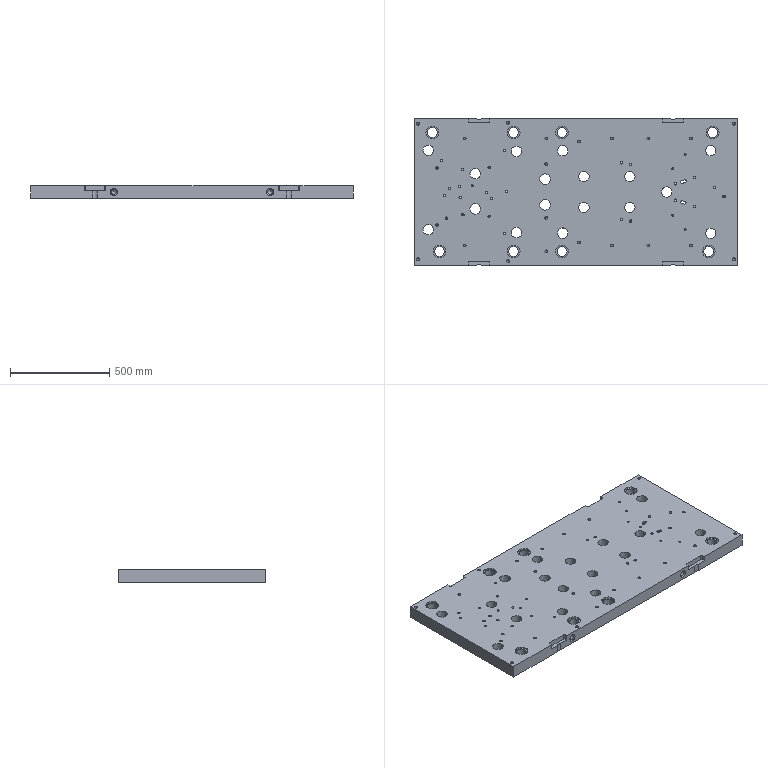Part | NX | features solid 2 | 1 solid | 601 faces | box 1630 x 740 x 65 mm | volume 71587254 mm3 | cylinder 316 | cone 157 | plane 122 | spline 6 | commonest cylinder face diameters 10 x56 8.5 x39 8.506 x26 12 x26 14.506 x22 10.506 x20